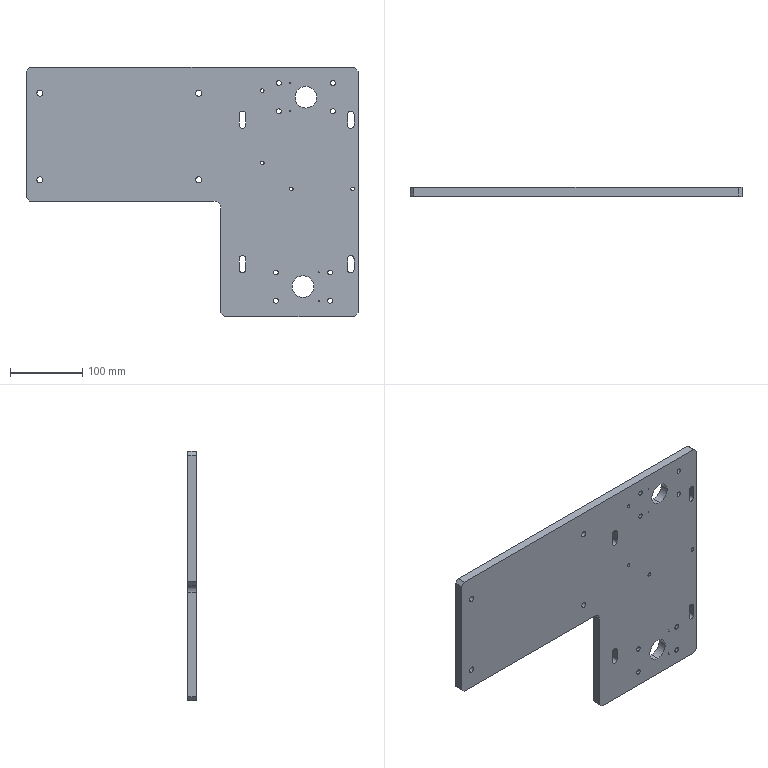Part | STEP file | PN_0009 | 1 solid | 102 faces | box 460 x 12 x 345 mm | volume 1349018 mm3 | cylinder 65 | plane 21 | cone 16 | commonest cylinder face diameters 5 x16 6.8 x16 9 x12 8 x8 8.5 x8 30 x4